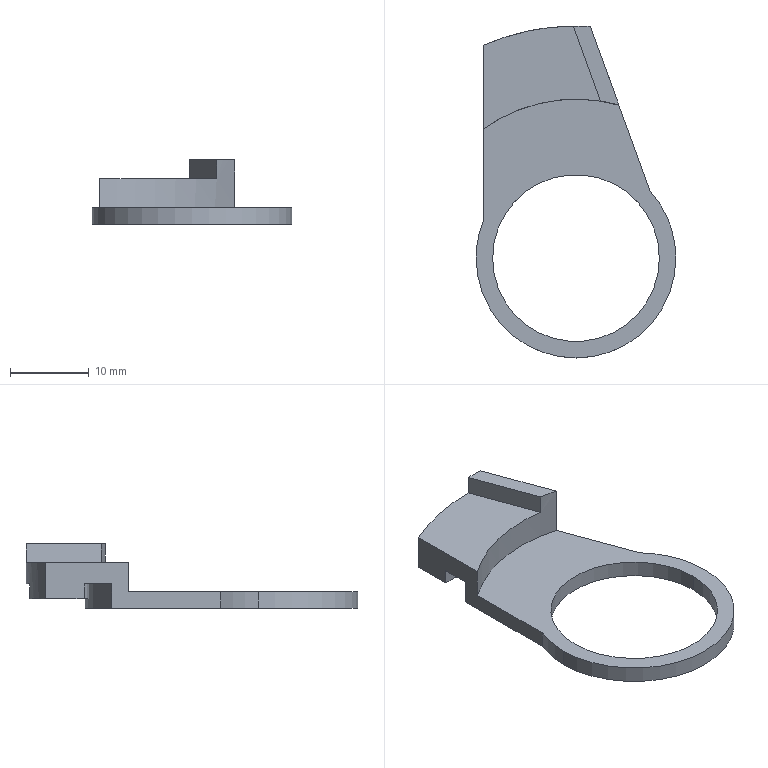Part | STEP file | A22NZ_H_01_LEVER | 1 solid | 21 faces | box 25.4 x 42.2 x 8.2 mm | volume 1285 mm3 | plane 11 | cylinder 10 | commonest cylinder face diameters 25.4 x3 7.5 x2 21.2 x2 40.4 x1 44 x1 59 x1
STEP:
#1=CARTESIAN_POINT('',(-4.25,25.26,-0.9));
#2=VERTEX_POINT('',#1);
#3=CARTESIAN_POINT('',(-10.035,22.11,-0.9));
#4=VERTEX_POINT('',#3);
#5=CARTESIAN_POINT('',(-8.,25.26,-0.9));
#6=DIRECTION('',(0.,0.,-1.));
#7=DIRECTION('',(-1.,0.,0.));
#8=AXIS2_PLACEMENT_3D('',#5,#6,#7);
#9=CIRCLE('',#8,3.75);
#10=EDGE_CURVE('',#2,#4,#9,.T.);
#11=ORIENTED_EDGE('',*,*,#10,.F.);
#12=CARTESIAN_POINT('',(-4.25,25.26,1.));
#13=VERTEX_POINT('',#12);
#14=CARTESIAN_POINT('',(-4.25,25.26,-0.9));
#15=DIRECTION('',(0.,0.,1.));
#16=VECTOR('',#15,1000.);
#17=LINE('',#14,#16);
#18=EDGE_CURVE('',#2,#13,#17,.T.);
#19=ORIENTED_EDGE('',*,*,#18,.T.);
#20=CARTESIAN_POINT('',(-10.035,22.11,1.));
#21=VERTEX_POINT('',#20);
#22=CARTESIAN_POINT('',(-8.,25.26,1.));
#23=DIRECTION('',(0.,0.,-1.));
#24=DIRECTION('',(-1.,0.,0.));
#25=AXIS2_PLACEMENT_3D('',#22,#23,#24);
#26=CIRCLE('',#25,3.75);
#27=EDGE_CURVE('',#13,#21,#26,.T.);
#28=ORIENTED_EDGE('',*,*,#27,.T.);
#29=CARTESIAN_POINT('',(-10.035,22.11,-0.9));
#30=DIRECTION('',(0.,0.,1.));
#31=VECTOR('',#30,1000.);
#32=LINE('',#29,#31);
#33=EDGE_CURVE('',#4,#21,#32,.T.);
#34=ORIENTED_EDGE('',*,*,#33,.F.);
#35=EDGE_LOOP('',(#11,#19,#28,#34));
#36=FACE_OUTER_BOUND('',#35,.T.);
#37=CARTESIAN_POINT('',(-8.,25.26,-0.9));
#38=DIRECTION('',(0.,0.,1.));
#39=DIRECTION('',(1.,0.,0.));
#40=AXIS2_PLACEMENT_3D('',#37,#38,#39);
#41=CYLINDRICAL_SURFACE('',#40,3.75);
#42=ADVANCED_FACE('',(#36),#41,.T.);
#43=CARTESIAN_POINT('',(10.6,0.,-2.1));
#44=VERTEX_POINT('',#43);
#45=CARTESIAN_POINT('',(-10.6,0.,-2.1));
#46=VERTEX_POINT('',#45);
#47=CARTESIAN_POINT('',(0.,0.,-2.1));
#48=DIRECTION('',(0.,0.,-1.));
#49=DIRECTION('',(-1.,0.,0.));
#50=AXIS2_PLACEMENT_3D('',#47,#48,#49);
#51=CIRCLE('',#50,10.6);
#52=EDGE_CURVE('',#44,#46,#51,.T.);
#53=ORIENTED_EDGE('',*,*,#52,.T.);
#54=CARTESIAN_POINT('',(-10.6,0.,0.));
#55=VERTEX_POINT('',#54);
#56=CARTESIAN_POINT('',(-10.6,0.,-2.1));
#57=DIRECTION('',(0.,0.,1.));
#58=VECTOR('',#57,1000.);
#59=LINE('',#56,#58);
#60=EDGE_CURVE('',#46,#55,#59,.T.);
#61=ORIENTED_EDGE('',*,*,#60,.T.);
#62=CARTESIAN_POINT('',(10.6,0.,0.));
#63=VERTEX_POINT('',#62);
#64=CARTESIAN_POINT('',(0.,0.,0.));
#65=DIRECTION('',(0.,0.,-1.));
#66=DIRECTION('',(-1.,0.,0.));
#67=AXIS2_PLACEMENT_3D('',#64,#65,#66);
#68=CIRCLE('',#67,10.6);
#69=EDGE_CURVE('',#63,#55,#68,.T.);
#70=ORIENTED_EDGE('',*,*,#69,.F.);
#71=CARTESIAN_POINT('',(10.6,0.,-2.1));
#72=DIRECTION('',(0.,0.,1.));
#73=VECTOR('',#72,1000.);
#74=LINE('',#71,#73);
#75=EDGE_CURVE('',#44,#63,#74,.T.);
#76=ORIENTED_EDGE('',*,*,#75,.F.);
#77=EDGE_LOOP('',(#53,#61,#70,#76));
#78=FACE_OUTER_BOUND('',#77,.T.);
#79=CARTESIAN_POINT('',(0.,0.,-2.1));
#80=DIRECTION('',(0.,0.,1.));
#81=DIRECTION('',(1.,0.,0.));
#82=AXIS2_PLACEMENT_3D('',#79,#80,#81);
#83=CYLINDRICAL_SURFACE('',#82,10.6);
#84=ADVANCED_FACE('',(#78),#83,.F.);
#85=CARTESIAN_POINT('',(-12.7,0.,-2.1));
#86=VERTEX_POINT('',#85);
#87=CARTESIAN_POINT('',(-11.78,4.746,-2.1));
#88=VERTEX_POINT('',#87);
#89=CARTESIAN_POINT('',(0.,0.,-2.1));
#90=DIRECTION('',(0.,0.,-1.));
#91=DIRECTION('',(-1.,0.,0.));
#92=AXIS2_PLACEMENT_3D('',#89,#90,#91);
#93=CIRCLE('',#92,12.7);
#94=EDGE_CURVE('',#86,#88,#93,.T.);
#95=ORIENTED_EDGE('',*,*,#94,.F.);
#96=CARTESIAN_POINT('',(-12.7,0.,0.));
#97=VERTEX_POINT('',#96);
#98=CARTESIAN_POINT('',(-12.7,0.,-2.1));
#99=DIRECTION('',(0.,0.,1.));
#100=VECTOR('',#99,1000.);
#101=LINE('',#98,#100);
#102=EDGE_CURVE('',#86,#97,#101,.T.);
#103=ORIENTED_EDGE('',*,*,#102,.T.);
#104=CARTESIAN_POINT('',(-11.78,4.746,0.));
#105=VERTEX_POINT('',#104);
#106=CARTESIAN_POINT('',(0.,0.,0.));
#107=DIRECTION('',(0.,0.,-1.));
#108=DIRECTION('',(-1.,0.,0.));
#109=AXIS2_PLACEMENT_3D('',#106,#107,#108);
#110=CIRCLE('',#109,12.7);
#111=EDGE_CURVE('',#97,#105,#110,.T.);
#112=ORIENTED_EDGE('',*,*,#111,.T.);
#113=CARTESIAN_POINT('',(-11.78,4.746,-2.1));
#114=DIRECTION('',(0.,0.,1.));
#115=VECTOR('',#114,1000.);
#116=LINE('',#113,#115);
#117=EDGE_CURVE('',#88,#105,#116,.T.);
#118=ORIENTED_EDGE('',*,*,#117,.F.);
#119=EDGE_LOOP('',(#95,#103,#112,#118));
#120=FACE_OUTER_BOUND('',#119,.T.);
#121=CARTESIAN_POINT('',(0.,0.,-2.1));
#122=DIRECTION('',(0.,0.,1.));
#123=DIRECTION('',(1.,0.,0.));
#124=AXIS2_PLACEMENT_3D('',#121,#122,#123);
#125=CYLINDRICAL_SURFACE('',#124,12.7);
#126=ADVANCED_FACE('',(#120),#125,.T.);
#127=ORIENTED_EDGE('',*,*,#102,.F.);
#128=CARTESIAN_POINT('',(12.7,0.,-2.1));
#129=VERTEX_POINT('',#128);
#130=CARTESIAN_POINT('',(0.,0.,-2.1));
#131=DIRECTION('',(0.,0.,-1.));
#132=DIRECTION('',(-1.,0.,0.));
#133=AXIS2_PLACEMENT_3D('',#130,#131,#132);
#134=CIRCLE('',#133,12.7);
#135=EDGE_CURVE('',#129,#86,#134,.T.);
#136=ORIENTED_EDGE('',*,*,#135,.F.);
#137=CARTESIAN_POINT('',(12.7,0.,0.));
#138=VERTEX_POINT('',#137);
#139=CARTESIAN_POINT('',(12.7,0.,-2.1));
#140=DIRECTION('',(0.,0.,1.));
#141=VECTOR('',#140,1000.);
#142=LINE('',#139,#141);
#143=EDGE_CURVE('',#129,#138,#142,.T.);
#144=ORIENTED_EDGE('',*,*,#143,.T.);
#145=CARTESIAN_POINT('',(0.,0.,0.));
#146=DIRECTION('',(0.,0.,-1.));
#147=DIRECTION('',(-1.,0.,0.));
#148=AXIS2_PLACEMENT_3D('',#145,#146,#147);
#149=CIRCLE('',#148,12.7);
#150=EDGE_CURVE('',#138,#97,#149,.T.);
#151=ORIENTED_EDGE('',*,*,#150,.T.);
#152=EDGE_LOOP('',(#127,#136,#144,#151));
#153=FACE_OUTER_BOUND('',#152,.T.);
#154=CARTESIAN_POINT('',(0.,0.,-2.1));
#155=DIRECTION('',(0.,0.,1.));
#156=DIRECTION('',(1.,0.,0.));
#157=AXIS2_PLACEMENT_3D('',#154,#155,#156);
#158=CYLINDRICAL_SURFACE('',#157,12.7);
#159=ADVANCED_FACE('',(#153),#158,.T.);
#160=CARTESIAN_POINT('',(-11.78,22.11,1.));
#161=VERTEX_POINT('',#160);
#162=CARTESIAN_POINT('',(-10.035,22.11,1.));
#163=DIRECTION('',(-1.,0.,0.));
#164=VECTOR('',#163,1000.);
#165=LINE('',#162,#164);
#166=EDGE_CURVE('',#21,#161,#165,.T.);
#167=ORIENTED_EDGE('',*,*,#166,.F.);
#168=ORIENTED_EDGE('',*,*,#27,.F.);
#169=CARTESIAN_POINT('',(-5.25,27.81,1.));
#170=VERTEX_POINT('',#169);
#171=CARTESIAN_POINT('',(-8.,25.26,1.));
#172=DIRECTION('',(0.,0.,-1.));
#173=DIRECTION('',(-1.,0.,0.));
#174=AXIS2_PLACEMENT_3D('',#171,#172,#173);
#175=CIRCLE('',#174,3.75);
#176=EDGE_CURVE('',#170,#13,#175,.T.);
#177=ORIENTED_EDGE('',*,*,#176,.F.);
#178=CARTESIAN_POINT('',(-5.25,29.029,1.));
#179=VERTEX_POINT('',#178);
#180=CARTESIAN_POINT('',(-5.25,27.81,1.));
#181=DIRECTION('',(0.,-1.,0.));
#182=VECTOR('',#181,1000.);
#183=LINE('',#180,#182);
#184=EDGE_CURVE('',#179,#170,#183,.T.);
#185=ORIENTED_EDGE('',*,*,#184,.F.);
#186=CARTESIAN_POINT('',(1.816,29.444,1.));
#187=VERTEX_POINT('',#186);
#188=CARTESIAN_POINT('',(0.,0.,1.));
#189=DIRECTION('',(0.,0.,1.));
#190=DIRECTION('',(1.,0.,0.));
#191=AXIS2_PLACEMENT_3D('',#188,#189,#190);
#192=CIRCLE('',#191,29.5);
#193=EDGE_CURVE('',#187,#179,#192,.T.);
#194=ORIENTED_EDGE('',*,*,#193,.F.);
#195=CARTESIAN_POINT('',(4.711,21.49,1.));
#196=VERTEX_POINT('',#195);
#197=CARTESIAN_POINT('',(5.454,19.45,1.));
#198=DIRECTION('',(-0.342,0.9397,0.));
#199=VECTOR('',#198,1000.);
#200=LINE('',#197,#199);
#201=EDGE_CURVE('',#196,#187,#200,.T.);
#202=ORIENTED_EDGE('',*,*,#201,.F.);
#203=CARTESIAN_POINT('',(-11.78,18.58,1.));
#204=VERTEX_POINT('',#203);
#205=CARTESIAN_POINT('',(0.,0.,1.));
#206=DIRECTION('',(0.,0.,1.));
#207=DIRECTION('',(1.,0.,0.));
#208=AXIS2_PLACEMENT_3D('',#205,#206,#207);
#209=CIRCLE('',#208,22.);
#210=EDGE_CURVE('',#196,#204,#209,.T.);
#211=ORIENTED_EDGE('',*,*,#210,.T.);
#212=CARTESIAN_POINT('',(-11.78,18.58,1.));
#213=DIRECTION('',(0.,1.,0.));
#214=VECTOR('',#213,1000.);
#215=LINE('',#212,#214);
#216=EDGE_CURVE('',#204,#161,#215,.T.);
#217=ORIENTED_EDGE('',*,*,#216,.T.);
#218=EDGE_LOOP('',(#167,#168,#177,#185,#194,#202,#211,#217));
#219=FACE_OUTER_BOUND('',#218,.T.);
#220=CARTESIAN_POINT('',(0.,0.,1.));
#221=DIRECTION('',(0.,0.,1.));
#222=DIRECTION('',(1.,0.,0.));
#223=AXIS2_PLACEMENT_3D('',#220,#221,#222);
#224=PLANE('',#223);
#225=ADVANCED_FACE('',(#219),#224,.F.);
#226=CARTESIAN_POINT('',(-11.78,18.58,-2.1));
#227=VERTEX_POINT('',#226);
#228=CARTESIAN_POINT('',(-11.78,18.58,-2.1));
#229=DIRECTION('',(0.,0.,1.));
#230=VECTOR('',#229,1000.);
#231=LINE('',#228,#230);
#232=EDGE_CURVE('',#227,#204,#231,.T.);
#233=ORIENTED_EDGE('',*,*,#232,.T.);
#234=ORIENTED_EDGE('',*,*,#210,.F.);
#235=CARTESIAN_POINT('',(4.711,21.49,-2.1));
#236=VERTEX_POINT('',#235);
#237=CARTESIAN_POINT('',(4.711,21.49,-2.1));
#238=DIRECTION('',(0.,0.,1.));
#239=VECTOR('',#238,1000.);
#240=LINE('',#237,#239);
#241=EDGE_CURVE('',#236,#196,#240,.T.);
#242=ORIENTED_EDGE('',*,*,#241,.F.);
#243=CARTESIAN_POINT('',(0.,0.,-2.1));
#244=DIRECTION('',(0.,0.,-1.));
#245=DIRECTION('',(1.,0.,0.));
#246=AXIS2_PLACEMENT_3D('',#243,#244,#245);
#247=CIRCLE('',#246,22.);
#248=EDGE_CURVE('',#227,#236,#247,.T.);
#249=ORIENTED_EDGE('',*,*,#248,.F.);
#250=EDGE_LOOP('',(#233,#234,#242,#249));
#251=FACE_OUTER_BOUND('',#250,.T.);
#252=CARTESIAN_POINT('',(0.,0.,-2.1));
#253=DIRECTION('',(0.,0.,1.));
#254=DIRECTION('',(1.,0.,0.));
#255=AXIS2_PLACEMENT_3D('',#252,#253,#254);
#256=CYLINDRICAL_SURFACE('',#255,22.);
#257=ADVANCED_FACE('',(#251),#256,.T.);
#258=CARTESIAN_POINT('',(-11.78,16.409,3.7));
#259=VERTEX_POINT('',#258);
#260=CARTESIAN_POINT('',(3.142,19.954,3.7));
#261=VERTEX_POINT('',#260);
#262=CARTESIAN_POINT('',(0.,0.,3.7));
#263=DIRECTION('',(0.,0.,-1.));
#264=DIRECTION('',(1.,0.,0.));
#265=AXIS2_PLACEMENT_3D('',#262,#263,#264);
#266=CIRCLE('',#265,20.2);
#267=EDGE_CURVE('',#259,#261,#266,.T.);
#268=ORIENTED_EDGE('',*,*,#267,.T.);
#269=CARTESIAN_POINT('',(-0.332,29.498,3.7));
#270=VERTEX_POINT('',#269);
#271=CARTESIAN_POINT('',(9.187,3.344,3.7));
#272=DIRECTION('',(-0.342,0.9397,0.));
#273=VECTOR('',#272,1000.);
#274=LINE('',#271,#273);
#275=EDGE_CURVE('',#261,#270,#274,.T.);
#276=ORIENTED_EDGE('',*,*,#275,.T.);
#277=CARTESIAN_POINT('',(-11.78,27.046,3.7));
#278=VERTEX_POINT('',#277);
#279=CARTESIAN_POINT('',(0.,0.,3.7));
#280=DIRECTION('',(0.,0.,-1.));
#281=DIRECTION('',(1.,0.,0.));
#282=AXIS2_PLACEMENT_3D('',#279,#280,#281);
#283=CIRCLE('',#282,29.5);
#284=EDGE_CURVE('',#278,#270,#283,.T.);
#285=ORIENTED_EDGE('',*,*,#284,.F.);
#286=CARTESIAN_POINT('',(-11.78,16.409,3.7));
#287=DIRECTION('',(0.,-1.,0.));
#288=VECTOR('',#287,1000.);
#289=LINE('',#286,#288);
#290=EDGE_CURVE('',#278,#259,#289,.T.);
#291=ORIENTED_EDGE('',*,*,#290,.T.);
#292=EDGE_LOOP('',(#268,#276,#285,#291));
#293=FACE_OUTER_BOUND('',#292,.T.);
#294=CARTESIAN_POINT('',(0.,0.,3.7));
#295=DIRECTION('',(0.,0.,1.));
#296=DIRECTION('',(1.,0.,0.));
#297=AXIS2_PLACEMENT_3D('',#294,#295,#296);
#298=PLANE('',#297);
#299=ADVANCED_FACE('',(#293),#298,.T.);
#300=ORIENTED_EDGE('',*,*,#69,.T.);
#301=CARTESIAN_POINT('',(0.,0.,0.));
#302=DIRECTION('',(0.,0.,-1.));
#303=DIRECTION('',(-1.,0.,0.));
#304=AXIS2_PLACEMENT_3D('',#301,#302,#303);
#305=CIRCLE('',#304,10.6);
#306=EDGE_CURVE('',#55,#63,#305,.T.);
#307=ORIENTED_EDGE('',*,*,#306,.T.);
#308=EDGE_LOOP('',(#300,#307));
#309=FACE_BOUND('',#308,.T.);
#310=CARTESIAN_POINT('',(-11.78,16.409,0.));
#311=VERTEX_POINT('',#310);
#312=CARTESIAN_POINT('',(5.454,19.45,0.));
#313=VERTEX_POINT('',#312);
#314=CARTESIAN_POINT('',(0.,0.,0.));
#315=DIRECTION('',(0.,0.,-1.));
#316=DIRECTION('',(1.,0.,0.));
#317=AXIS2_PLACEMENT_3D('',#314,#315,#316);
#318=CIRCLE('',#317,20.2);
#319=EDGE_CURVE('',#311,#313,#318,.T.);
#320=ORIENTED_EDGE('',*,*,#319,.F.);
#321=CARTESIAN_POINT('',(-11.78,4.746,0.));
#322=DIRECTION('',(0.,1.,0.));
#323=VECTOR('',#322,1000.);
#324=LINE('',#321,#323);
#325=EDGE_CURVE('',#105,#311,#324,.T.);
#326=ORIENTED_EDGE('',*,*,#325,.F.);
#327=ORIENTED_EDGE('',*,*,#111,.F.);
#328=ORIENTED_EDGE('',*,*,#150,.F.);
#329=CARTESIAN_POINT('',(9.441,8.495,0.));
#330=VERTEX_POINT('',#329);
#331=CARTESIAN_POINT('',(0.,0.,0.));
#332=DIRECTION('',(0.,0.,-1.));
#333=DIRECTION('',(-1.,0.,0.));
#334=AXIS2_PLACEMENT_3D('',#331,#332,#333);
#335=CIRCLE('',#334,12.7);
#336=EDGE_CURVE('',#330,#138,#335,.T.);
#337=ORIENTED_EDGE('',*,*,#336,.F.);
#338=CARTESIAN_POINT('',(9.441,8.495,0.));
#339=DIRECTION('',(0.342,-0.9397,0.));
#340=VECTOR('',#339,1000.);
#341=LINE('',#338,#340);
#342=EDGE_CURVE('',#313,#330,#341,.T.);
#343=ORIENTED_EDGE('',*,*,#342,.F.);
#344=EDGE_LOOP('',(#320,#326,#327,#328,#337,#343));
#345=FACE_OUTER_BOUND('',#344,.T.);
#346=CARTESIAN_POINT('',(0.,0.,0.));
#347=DIRECTION('',(0.,0.,-1.));
#348=DIRECTION('',(-1.,0.,0.));
#349=AXIS2_PLACEMENT_3D('',#346,#347,#348);
#350=PLANE('',#349);
#351=ADVANCED_FACE('',(#309,#345),#350,.F.);
#352=CARTESIAN_POINT('',(9.441,8.495,-2.1));
#353=VERTEX_POINT('',#352);
#354=CARTESIAN_POINT('',(0.,0.,-2.1));
#355=DIRECTION('',(0.,0.,-1.));
#356=DIRECTION('',(-1.,0.,0.));
#357=AXIS2_PLACEMENT_3D('',#354,#355,#356);
#358=CIRCLE('',#357,12.7);
#359=EDGE_CURVE('',#353,#129,#358,.T.);
#360=ORIENTED_EDGE('',*,*,#359,.T.);
#361=ORIENTED_EDGE('',*,*,#135,.T.);
#362=ORIENTED_EDGE('',*,*,#94,.T.);
#363=CARTESIAN_POINT('',(-11.78,4.746,-2.1));
#364=DIRECTION('',(0.,1.,0.));
#365=VECTOR('',#364,1000.);
#366=LINE('',#363,#365);
#367=EDGE_CURVE('',#88,#227,#366,.T.);
#368=ORIENTED_EDGE('',*,*,#367,.T.);
#369=ORIENTED_EDGE('',*,*,#248,.T.);
#370=CARTESIAN_POINT('',(9.441,8.495,-2.1));
#371=DIRECTION('',(0.342,-0.9397,0.));
#372=VECTOR('',#371,1000.);
#373=LINE('',#370,#372);
#374=EDGE_CURVE('',#236,#353,#373,.T.);
#375=ORIENTED_EDGE('',*,*,#374,.T.);
#376=EDGE_LOOP('',(#360,#361,#362,#368,#369,#375));
#377=FACE_OUTER_BOUND('',#376,.T.);
#378=ORIENTED_EDGE('',*,*,#52,.F.);
#379=CARTESIAN_POINT('',(0.,0.,-2.1));
#380=DIRECTION('',(0.,0.,-1.));
#381=DIRECTION('',(-1.,0.,0.));
#382=AXIS2_PLACEMENT_3D('',#379,#380,#381);
#383=CIRCLE('',#382,10.6);
#384=EDGE_CURVE('',#46,#44,#383,.T.);
#385=ORIENTED_EDGE('',*,*,#384,.F.);
#386=EDGE_LOOP('',(#378,#385));
#387=FACE_BOUND('',#386,.T.);
#388=CARTESIAN_POINT('',(0.,0.,-2.1));
#389=DIRECTION('',(0.,0.,-1.));
#390=DIRECTION('',(-1.,0.,0.));
#391=AXIS2_PLACEMENT_3D('',#388,#389,#390);
#392=PLANE('',#391);
#393=ADVANCED_FACE('',(#377,#387),#392,.T.);
#394=ORIENTED_EDGE('',*,*,#143,.F.);
#395=ORIENTED_EDGE('',*,*,#359,.F.);
#396=CARTESIAN_POINT('',(9.441,8.495,-2.1));
#397=DIRECTION('',(0.,0.,1.));
#398=VECTOR('',#397,1000.);
#399=LINE('',#396,#398);
#400=EDGE_CURVE('',#353,#330,#399,.T.);
#401=ORIENTED_EDGE('',*,*,#400,.T.);
#402=ORIENTED_EDGE('',*,*,#336,.T.);
#403=EDGE_LOOP('',(#394,#395,#401,#402));
#404=FACE_OUTER_BOUND('',#403,.T.);
#405=CARTESIAN_POINT('',(0.,0.,-2.1));
#406=DIRECTION('',(0.,0.,1.));
#407=DIRECTION('',(1.,0.,0.));
#408=AXIS2_PLACEMENT_3D('',#405,#406,#407);
#409=CYLINDRICAL_SURFACE('',#408,12.7);
#410=ADVANCED_FACE('',(#404),#409,.T.);
#411=ORIENTED_EDGE('',*,*,#325,.T.);
#412=CARTESIAN_POINT('',(-11.78,16.409,3.7));
#413=DIRECTION('',(0.,0.,-1.));
#414=VECTOR('',#413,1000.);
#415=LINE('',#412,#414);
#416=EDGE_CURVE('',#259,#311,#415,.T.);
#417=ORIENTED_EDGE('',*,*,#416,.F.);
#418=ORIENTED_EDGE('',*,*,#290,.F.);
#419=CARTESIAN_POINT('',(-11.78,27.046,-0.9));
#420=VERTEX_POINT('',#419);
#421=CARTESIAN_POINT('',(-11.78,27.046,21.633));
#422=DIRECTION('',(0.,0.,-1.));
#423=VECTOR('',#422,1000.);
#424=LINE('',#421,#423);
#425=EDGE_CURVE('',#278,#420,#424,.T.);
#426=ORIENTED_EDGE('',*,*,#425,.T.);
#427=CARTESIAN_POINT('',(-11.78,22.11,-0.9));
#428=VERTEX_POINT('',#427);
#429=CARTESIAN_POINT('',(-11.78,22.11,-0.9));
#430=DIRECTION('',(0.,1.,0.));
#431=VECTOR('',#430,1000.);
#432=LINE('',#429,#431);
#433=EDGE_CURVE('',#428,#420,#432,.T.);
#434=ORIENTED_EDGE('',*,*,#433,.F.);
#435=CARTESIAN_POINT('',(-11.78,22.11,-0.9));
#436=DIRECTION('',(0.,0.,1.));
#437=VECTOR('',#436,1000.);
#438=LINE('',#435,#437);
#439=EDGE_CURVE('',#428,#161,#438,.T.);
#440=ORIENTED_EDGE('',*,*,#439,.T.);
#441=ORIENTED_EDGE('',*,*,#216,.F.);
#442=ORIENTED_EDGE('',*,*,#232,.F.);
#443=ORIENTED_EDGE('',*,*,#367,.F.);
#444=ORIENTED_EDGE('',*,*,#117,.T.);
#445=EDGE_LOOP('',(#411,#417,#418,#426,#434,#440,#441,#442,#443,#444));
#446=FACE_OUTER_BOUND('',#445,.T.);
#447=CARTESIAN_POINT('',(-11.78,4.746,-2.1));
#448=DIRECTION('',(1.,0.,0.));
#449=DIRECTION('',(0.,0.,-1.));
#450=AXIS2_PLACEMENT_3D('',#447,#448,#449);
#451=PLANE('',#450);
#452=ADVANCED_FACE('',(#446),#451,.F.);
#453=ORIENTED_EDGE('',*,*,#241,.T.);
#454=ORIENTED_EDGE('',*,*,#201,.T.);
#455=CARTESIAN_POINT('',(1.816,29.444,6.1));
#456=VERTEX_POINT('',#455);
#457=CARTESIAN_POINT('',(1.816,29.444,6.1));
#458=DIRECTION('',(0.,0.,-1.));
#459=VECTOR('',#458,1000.);
#460=LINE('',#457,#459);
#461=EDGE_CURVE('',#456,#187,#460,.T.);
#462=ORIENTED_EDGE('',*,*,#461,.F.);
#463=CARTESIAN_POINT('',(5.454,19.45,6.1));
#464=VERTEX_POINT('',#463);
#465=CARTESIAN_POINT('',(5.454,19.45,6.1));
#466=DIRECTION('',(-0.342,0.9397,0.));
#467=VECTOR('',#466,1000.);
#468=LINE('',#465,#467);
#469=EDGE_CURVE('',#464,#456,#468,.T.);
#470=ORIENTED_EDGE('',*,*,#469,.F.);
#471=CARTESIAN_POINT('',(5.454,19.45,3.7));
#472=DIRECTION('',(0.,0.,-1.));
#473=VECTOR('',#472,1000.);
#474=LINE('',#471,#473);
#475=EDGE_CURVE('',#464,#313,#474,.T.);
#476=ORIENTED_EDGE('',*,*,#475,.T.);
#477=ORIENTED_EDGE('',*,*,#342,.T.);
#478=ORIENTED_EDGE('',*,*,#400,.F.);
#479=ORIENTED_EDGE('',*,*,#374,.F.);
#480=EDGE_LOOP('',(#453,#454,#462,#470,#476,#477,#478,#479));
#481=FACE_OUTER_BOUND('',#480,.T.);
#482=CARTESIAN_POINT('',(9.441,8.495,-2.1));
#483=DIRECTION('',(-0.9397,-0.342,0.));
#484=DIRECTION('',(0.342,-0.9397,0.));
#485=AXIS2_PLACEMENT_3D('',#482,#483,#484);
#486=PLANE('',#485);
#487=ADVANCED_FACE('',(#481),#486,.F.);
#488=ORIENTED_EDGE('',*,*,#60,.F.);
#489=ORIENTED_EDGE('',*,*,#384,.T.);
#490=ORIENTED_EDGE('',*,*,#75,.T.);
#491=ORIENTED_EDGE('',*,*,#306,.F.);
#492=EDGE_LOOP('',(#488,#489,#490,#491));
#493=FACE_OUTER_BOUND('',#492,.T.);
#494=CARTESIAN_POINT('',(0.,0.,-2.1));
#495=DIRECTION('',(0.,0.,1.));
#496=DIRECTION('',(1.,0.,0.));
#497=AXIS2_PLACEMENT_3D('',#494,#495,#496);
#498=CYLINDRICAL_SURFACE('',#497,10.6);
#499=ADVANCED_FACE('',(#493),#498,.F.);
#500=ORIENTED_EDGE('',*,*,#475,.F.);
#501=CARTESIAN_POINT('',(3.142,19.954,6.1));
#502=VERTEX_POINT('',#501);
#503=CARTESIAN_POINT('',(0.,0.,6.1));
#504=DIRECTION('',(0.,0.,-1.));
#505=DIRECTION('',(1.,0.,0.));
#506=AXIS2_PLACEMENT_3D('',#503,#504,#505);
#507=CIRCLE('',#506,20.2);
#508=EDGE_CURVE('',#502,#464,#507,.T.);
#509=ORIENTED_EDGE('',*,*,#508,.F.);
#510=CARTESIAN_POINT('',(3.142,19.954,6.1));
#511=DIRECTION('',(0.,0.,-1.));
#512=VECTOR('',#511,1000.);
#513=LINE('',#510,#512);
#514=EDGE_CURVE('',#502,#261,#513,.T.);
#515=ORIENTED_EDGE('',*,*,#514,.T.);
#516=ORIENTED_EDGE('',*,*,#267,.F.);
#517=ORIENTED_EDGE('',*,*,#416,.T.);
#518=ORIENTED_EDGE('',*,*,#319,.T.);
#519=EDGE_LOOP('',(#500,#509,#515,#516,#517,#518));
#520=FACE_OUTER_BOUND('',#519,.T.);
#521=CARTESIAN_POINT('',(0.,0.,3.7));
#522=DIRECTION('',(0.,0.,-1.));
#523=DIRECTION('',(-1.,0.,0.));
#524=AXIS2_PLACEMENT_3D('',#521,#522,#523);
#525=CYLINDRICAL_SURFACE('',#524,20.2);
#526=ADVANCED_FACE('',(#520),#525,.F.);
#527=CARTESIAN_POINT('',(-0.332,29.498,6.1));
#528=VERTEX_POINT('',#527);
#529=CARTESIAN_POINT('',(-0.332,29.498,6.1));
#530=DIRECTION('',(0.,0.,-1.));
#531=VECTOR('',#530,1000.);
#532=LINE('',#529,#531);
#533=EDGE_CURVE('',#528,#270,#532,.T.);
#534=ORIENTED_EDGE('',*,*,#533,.T.);
#535=ORIENTED_EDGE('',*,*,#275,.F.);
#536=ORIENTED_EDGE('',*,*,#514,.F.);
#537=CARTESIAN_POINT('',(3.142,19.954,6.1));
#538=DIRECTION('',(0.342,-0.9397,0.));
#539=VECTOR('',#538,1000.);
#540=LINE('',#537,#539);
#541=EDGE_CURVE('',#528,#502,#540,.T.);
#542=ORIENTED_EDGE('',*,*,#541,.F.);
#543=EDGE_LOOP('',(#534,#535,#536,#542));
#544=FACE_OUTER_BOUND('',#543,.T.);
#545=CARTESIAN_POINT('',(3.142,19.954,6.1));
#546=DIRECTION('',(0.9397,0.342,0.));
#547=DIRECTION('',(-0.342,0.9397,0.));
#548=AXIS2_PLACEMENT_3D('',#545,#546,#547);
#549=PLANE('',#548);
#550=ADVANCED_FACE('',(#544),#549,.F.);
#551=ORIENTED_EDGE('',*,*,#461,.T.);
#552=ORIENTED_EDGE('',*,*,#193,.T.);
#553=CARTESIAN_POINT('',(-5.25,29.029,-0.9));
#554=VERTEX_POINT('',#553);
#555=CARTESIAN_POINT('',(-5.25,29.029,-0.9));
#556=DIRECTION('',(0.,0.,1.));
#557=VECTOR('',#556,1000.);
#558=LINE('',#555,#557);
#559=EDGE_CURVE('',#554,#179,#558,.T.);
#560=ORIENTED_EDGE('',*,*,#559,.F.);
#561=CARTESIAN_POINT('',(0.,0.,-0.9));
#562=DIRECTION('',(0.,0.,-1.));
#563=DIRECTION('',(-1.,0.,0.));
#564=AXIS2_PLACEMENT_3D('',#561,#562,#563);
#565=CIRCLE('',#564,29.5);
#566=EDGE_CURVE('',#420,#554,#565,.T.);
#567=ORIENTED_EDGE('',*,*,#566,.F.);
#568=ORIENTED_EDGE('',*,*,#425,.F.);
#569=ORIENTED_EDGE('',*,*,#284,.T.);
#570=ORIENTED_EDGE('',*,*,#533,.F.);
#571=CARTESIAN_POINT('',(0.,0.,6.1));
#572=DIRECTION('',(0.,0.,1.));
#573=DIRECTION('',(1.,0.,0.));
#574=AXIS2_PLACEMENT_3D('',#571,#572,#573);
#575=CIRCLE('',#574,29.5);
#576=EDGE_CURVE('',#456,#528,#575,.T.);
#577=ORIENTED_EDGE('',*,*,#576,.F.);
#578=EDGE_LOOP('',(#551,#552,#560,#567,#568,#569,#570,#577));
#579=FACE_OUTER_BOUND('',#578,.T.);
#580=CARTESIAN_POINT('',(0.,0.,6.1));
#581=DIRECTION('',(0.,0.,-1.));
#582=DIRECTION('',(-1.,0.,0.));
#583=AXIS2_PLACEMENT_3D('',#580,#581,#582);
#584=CYLINDRICAL_SURFACE('',#583,29.5);
#585=ADVANCED_FACE('',(#579),#584,.T.);
#586=ORIENTED_EDGE('',*,*,#508,.T.);
#587=ORIENTED_EDGE('',*,*,#469,.T.);
#588=ORIENTED_EDGE('',*,*,#576,.T.);
#589=ORIENTED_EDGE('',*,*,#541,.T.);
#590=EDGE_LOOP('',(#586,#587,#588,#589));
#591=FACE_OUTER_BOUND('',#590,.T.);
#592=CARTESIAN_POINT('',(0.,0.,6.1));
#593=DIRECTION('',(0.,0.,1.));
#594=DIRECTION('',(1.,0.,0.));
#595=AXIS2_PLACEMENT_3D('',#592,#593,#594);
#596=PLANE('',#595);
#597=ADVANCED_FACE('',(#591),#596,.T.);
#598=ORIENTED_EDGE('',*,*,#18,.F.);
#599=CARTESIAN_POINT('',(-5.25,27.81,-0.9));
#600=VERTEX_POINT('',#599);
#601=CARTESIAN_POINT('',(-8.,25.26,-0.9));
#602=DIRECTION('',(0.,0.,-1.));
#603=DIRECTION('',(-1.,0.,0.));
#604=AXIS2_PLACEMENT_3D('',#601,#602,#603);
#605=CIRCLE('',#604,3.75);
#606=EDGE_CURVE('',#600,#2,#605,.T.);
#607=ORIENTED_EDGE('',*,*,#606,.F.);
#608=CARTESIAN_POINT('',(-5.25,27.81,-0.9));
#609=DIRECTION('',(0.,0.,1.));
#610=VECTOR('',#609,1000.);
#611=LINE('',#608,#610);
#612=EDGE_CURVE('',#600,#170,#611,.T.);
#613=ORIENTED_EDGE('',*,*,#612,.T.);
#614=ORIENTED_EDGE('',*,*,#176,.T.);
#615=EDGE_LOOP('',(#598,#607,#613,#614));
#616=FACE_OUTER_BOUND('',#615,.T.);
#617=CARTESIAN_POINT('',(-8.,25.26,-0.9));
#618=DIRECTION('',(0.,0.,1.));
#619=DIRECTION('',(1.,0.,0.));
#620=AXIS2_PLACEMENT_3D('',#617,#618,#619);
#621=CYLINDRICAL_SURFACE('',#620,3.75);
#622=ADVANCED_FACE('',(#616),#621,.T.);
#623=ORIENTED_EDGE('',*,*,#166,.T.);
#624=ORIENTED_EDGE('',*,*,#439,.F.);
#625=CARTESIAN_POINT('',(-10.035,22.11,-0.9));
#626=DIRECTION('',(-1.,0.,0.));
#627=VECTOR('',#626,1000.);
#628=LINE('',#625,#627);
#629=EDGE_CURVE('',#4,#428,#628,.T.);
#630=ORIENTED_EDGE('',*,*,#629,.F.);
#631=ORIENTED_EDGE('',*,*,#33,.T.);
#632=EDGE_LOOP('',(#623,#624,#630,#631));
#633=FACE_OUTER_BOUND('',#632,.T.);
#634=CARTESIAN_POINT('',(-10.035,22.11,-0.9));
#635=DIRECTION('',(0.,1.,0.));
#636=DIRECTION('',(0.,0.,1.));
#637=AXIS2_PLACEMENT_3D('',#634,#635,#636);
#638=PLANE('',#637);
#639=ADVANCED_FACE('',(#633),#638,.F.);
#640=ORIENTED_EDGE('',*,*,#184,.T.);
#641=ORIENTED_EDGE('',*,*,#612,.F.);
#642=CARTESIAN_POINT('',(-5.25,27.81,-0.9));
#643=DIRECTION('',(0.,-1.,0.));
#644=VECTOR('',#643,1000.);
#645=LINE('',#642,#644);
#646=EDGE_CURVE('',#554,#600,#645,.T.);
#647=ORIENTED_EDGE('',*,*,#646,.F.);
#648=ORIENTED_EDGE('',*,*,#559,.T.);
#649=EDGE_LOOP('',(#640,#641,#647,#648));
#650=FACE_OUTER_BOUND('',#649,.T.);
#651=CARTESIAN_POINT('',(-5.25,27.81,-0.9));
#652=DIRECTION('',(-1.,0.,0.));
#653=DIRECTION('',(0.,0.,1.));
#654=AXIS2_PLACEMENT_3D('',#651,#652,#653);
#655=PLANE('',#654);
#656=ADVANCED_FACE('',(#650),#655,.F.);
#657=ORIENTED_EDGE('',*,*,#606,.T.);
#658=ORIENTED_EDGE('',*,*,#10,.T.);
#659=ORIENTED_EDGE('',*,*,#629,.T.);
#660=ORIENTED_EDGE('',*,*,#433,.T.);
#661=ORIENTED_EDGE('',*,*,#566,.T.);
#662=ORIENTED_EDGE('',*,*,#646,.T.);
#663=EDGE_LOOP('',(#657,#658,#659,#660,#661,#662));
#664=FACE_OUTER_BOUND('',#663,.T.);
#665=CARTESIAN_POINT('',(-8.,25.26,-0.9));
#666=DIRECTION('',(0.,0.,-1.));
#667=DIRECTION('',(-1.,0.,0.));
#668=AXIS2_PLACEMENT_3D('',#665,#666,#667);
#669=PLANE('',#668);
#670=ADVANCED_FACE('',(#664),#669,.T.);
#671=CLOSED_SHELL('',(#42,#84,#126,#159,#225,#257,#299,#351,#393,#410,#452,#487,#499,#526,#550,#585,#597,#622,#639,#656,#670));
#672=MANIFOLD_SOLID_BREP('',#671);
#673=CARTESIAN_POINT('',(0.,0.,0.));
#674=DIRECTION('',(0.,0.,1.));
#675=DIRECTION('',(1.,0.,0.));
#676=AXIS2_PLACEMENT_3D('',#673,#674,#675);
#677=(LENGTH_UNIT()NAMED_UNIT(*)SI_UNIT(.MILLI.,.METRE.));
#678=UNCERTAINTY_MEASURE_WITH_UNIT(LENGTH_MEASURE(0.00001),#677,'','');
#679=(NAMED_UNIT(*)PLANE_ANGLE_UNIT()SI_UNIT($,.RADIAN.));
#680=(NAMED_UNIT(*)SI_UNIT($,.STERADIAN.)SOLID_ANGLE_UNIT());
#681=(GEOMETRIC_REPRESENTATION_CONTEXT(3)GLOBAL_UNCERTAINTY_ASSIGNED_CONTEXT((#678))GLOBAL_UNIT_ASSIGNED_CONTEXT((#677,#679,#680))REPRESENTATION_CONTEXT('',''));
#682=ADVANCED_BREP_SHAPE_REPRESENTATION('',(#672,#676),#681);